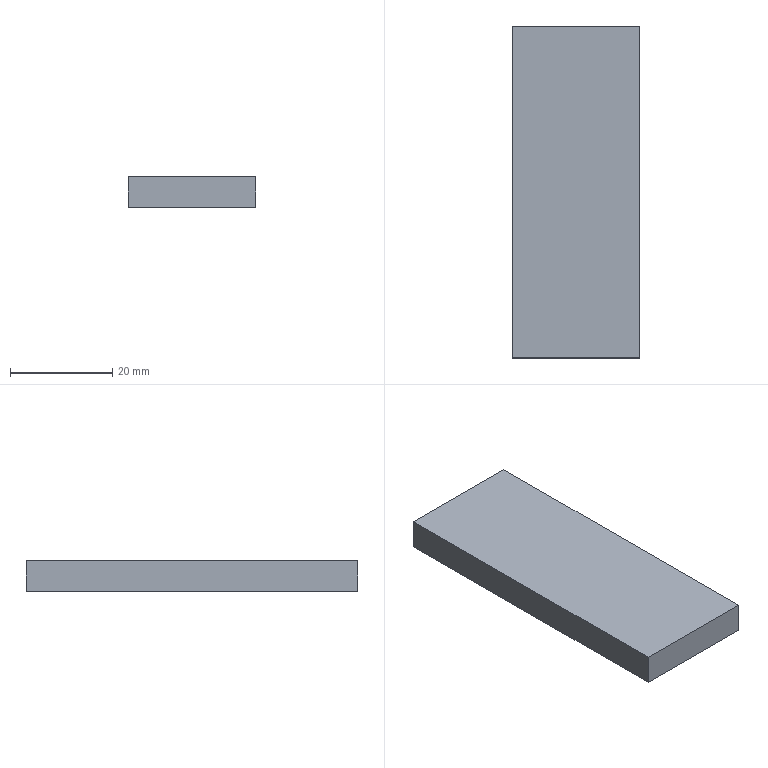Part | STEP file | 09-Steel plate 25x65x6 | 1 solid | 6 faces | box 25 x 65 x 6 mm | volume 9750 mm3 | plane 6
STEP:
#1=CARTESIAN_POINT('',(0.,0.,0.));
#2=DIRECTION('',(0.,0.,1.));
#3=DIRECTION('',(1.,0.,0.));
#4=AXIS2_PLACEMENT_3D('',#1,#2,#3);
#5=CARTESIAN_POINT('',(0.,0.,0.));
#6=VERTEX_POINT('',#5);
#7=CARTESIAN_POINT('',(0.,-65.,0.));
#8=VERTEX_POINT('',#7);
#9=CARTESIAN_POINT('',(0.,0.,0.));
#10=DIRECTION('',(0.,-1.,0.));
#11=VECTOR('',#10,1.);
#12=LINE('',#9,#11);
#13=CARTESIAN_POINT('',(0.,0.,6.));
#14=DIRECTION('',(1.,0.,0.));
#15=DIRECTION('',(0.,1.,0.));
#16=AXIS2_PLACEMENT_3D('',#13,#14,#15);
#17=PLANE('',#16);
#18=CARTESIAN_POINT('',(0.,-6.));
#19=DIRECTION('',(-1.,0.));
#20=VECTOR('',#19,1.);
#21=LINE('',#18,#20);
#22=(GEOMETRIC_REPRESENTATION_CONTEXT(2)PARAMETRIC_REPRESENTATION_CONTEXT()REPRESENTATION_CONTEXT('',''));
#23=DEFINITIONAL_REPRESENTATION('',(#21),#22);
#24=PCURVE('',#17,#23);
#25=CARTESIAN_POINT('',(0.,0.,0.));
#26=DIRECTION('',(0.,0.,1.));
#27=DIRECTION('',(1.,0.,0.));
#28=AXIS2_PLACEMENT_3D('',#25,#26,#27);
#29=PLANE('',#28);
#30=CARTESIAN_POINT('',(0.,0.));
#31=DIRECTION('',(0.,-1.));
#32=VECTOR('',#31,1.);
#33=LINE('',#30,#32);
#34=(GEOMETRIC_REPRESENTATION_CONTEXT(2)PARAMETRIC_REPRESENTATION_CONTEXT()REPRESENTATION_CONTEXT('',''));
#35=DEFINITIONAL_REPRESENTATION('',(#33),#34);
#36=PCURVE('',#29,#35);
#37=SURFACE_CURVE('',#12,(#24,#36),.PCURVE_S1.);
#38=EDGE_CURVE('',#6,#8,#37,.T.);
#39=ORIENTED_EDGE('',*,*,#38,.T.);
#40=CARTESIAN_POINT('',(0.,-65.,6.));
#41=VERTEX_POINT('',#40);
#42=CARTESIAN_POINT('',(0.,-65.,6.));
#43=DIRECTION('',(0.,0.,-1.));
#44=VECTOR('',#43,1.);
#45=LINE('',#42,#44);
#46=CARTESIAN_POINT('',(-65.,0.));
#47=DIRECTION('',(0.,-1.));
#48=VECTOR('',#47,1.);
#49=LINE('',#46,#48);
#50=(GEOMETRIC_REPRESENTATION_CONTEXT(2)PARAMETRIC_REPRESENTATION_CONTEXT()REPRESENTATION_CONTEXT('',''));
#51=DEFINITIONAL_REPRESENTATION('',(#49),#50);
#52=PCURVE('',#17,#51);
#53=CARTESIAN_POINT('',(0.,-65.,6.));
#54=DIRECTION('',(0.,1.,0.));
#55=DIRECTION('',(0.,0.,1.));
#56=AXIS2_PLACEMENT_3D('',#53,#54,#55);
#57=PLANE('',#56);
#58=CARTESIAN_POINT('',(0.,0.));
#59=DIRECTION('',(-1.,0.));
#60=VECTOR('',#59,1.);
#61=LINE('',#58,#60);
#62=(GEOMETRIC_REPRESENTATION_CONTEXT(2)PARAMETRIC_REPRESENTATION_CONTEXT()REPRESENTATION_CONTEXT('',''));
#63=DEFINITIONAL_REPRESENTATION('',(#61),#62);
#64=PCURVE('',#57,#63);
#65=SURFACE_CURVE('',#45,(#52,#64),.PCURVE_S1.);
#66=EDGE_CURVE('',#41,#8,#65,.T.);
#67=ORIENTED_EDGE('',*,*,#66,.F.);
#68=CARTESIAN_POINT('',(0.,0.,6.));
#69=VERTEX_POINT('',#68);
#70=CARTESIAN_POINT('',(0.,0.,6.));
#71=DIRECTION('',(0.,-1.,0.));
#72=VECTOR('',#71,1.);
#73=LINE('',#70,#72);
#74=CARTESIAN_POINT('',(0.,0.));
#75=DIRECTION('',(-1.,0.));
#76=VECTOR('',#75,1.);
#77=LINE('',#74,#76);
#78=(GEOMETRIC_REPRESENTATION_CONTEXT(2)PARAMETRIC_REPRESENTATION_CONTEXT()REPRESENTATION_CONTEXT('',''));
#79=DEFINITIONAL_REPRESENTATION('',(#77),#78);
#80=PCURVE('',#17,#79);
#81=CARTESIAN_POINT('',(0.,0.,6.));
#82=DIRECTION('',(0.,0.,1.));
#83=DIRECTION('',(1.,0.,0.));
#84=AXIS2_PLACEMENT_3D('',#81,#82,#83);
#85=PLANE('',#84);
#86=CARTESIAN_POINT('',(0.,0.));
#87=DIRECTION('',(0.,-1.));
#88=VECTOR('',#87,1.);
#89=LINE('',#86,#88);
#90=(GEOMETRIC_REPRESENTATION_CONTEXT(2)PARAMETRIC_REPRESENTATION_CONTEXT()REPRESENTATION_CONTEXT('',''));
#91=DEFINITIONAL_REPRESENTATION('',(#89),#90);
#92=PCURVE('',#85,#91);
#93=SURFACE_CURVE('',#73,(#80,#92),.PCURVE_S1.);
#94=EDGE_CURVE('',#69,#41,#93,.T.);
#95=ORIENTED_EDGE('',*,*,#94,.F.);
#96=CARTESIAN_POINT('',(0.,0.,6.));
#97=DIRECTION('',(0.,0.,-1.));
#98=VECTOR('',#97,1.);
#99=LINE('',#96,#98);
#100=CARTESIAN_POINT('',(0.,0.));
#101=DIRECTION('',(0.,-1.));
#102=VECTOR('',#101,1.);
#103=LINE('',#100,#102);
#104=(GEOMETRIC_REPRESENTATION_CONTEXT(2)PARAMETRIC_REPRESENTATION_CONTEXT()REPRESENTATION_CONTEXT('',''));
#105=DEFINITIONAL_REPRESENTATION('',(#103),#104);
#106=PCURVE('',#17,#105);
#107=CARTESIAN_POINT('',(0.,0.,6.));
#108=DIRECTION('',(0.,-1.,0.));
#109=DIRECTION('',(0.,0.,-1.));
#110=AXIS2_PLACEMENT_3D('',#107,#108,#109);
#111=PLANE('',#110);
#112=CARTESIAN_POINT('',(0.,0.));
#113=DIRECTION('',(1.,0.));
#114=VECTOR('',#113,1.);
#115=LINE('',#112,#114);
#116=(GEOMETRIC_REPRESENTATION_CONTEXT(2)PARAMETRIC_REPRESENTATION_CONTEXT()REPRESENTATION_CONTEXT('',''));
#117=DEFINITIONAL_REPRESENTATION('',(#115),#116);
#118=PCURVE('',#111,#117);
#119=SURFACE_CURVE('',#99,(#106,#118),.PCURVE_S1.);
#120=EDGE_CURVE('',#69,#6,#119,.T.);
#121=ORIENTED_EDGE('',*,*,#120,.T.);
#122=EDGE_LOOP('',(#39,#67,#95,#121));
#123=FACE_BOUND('',#122,.T.);
#124=ADVANCED_FACE('',(#123),#17,.F.);
#125=CARTESIAN_POINT('',(25.,-65.,0.));
#126=VERTEX_POINT('',#125);
#127=CARTESIAN_POINT('',(0.,-65.,0.));
#128=DIRECTION('',(1.,0.,0.));
#129=VECTOR('',#128,1.);
#130=LINE('',#127,#129);
#131=CARTESIAN_POINT('',(-6.,0.));
#132=DIRECTION('',(0.,1.));
#133=VECTOR('',#132,1.);
#134=LINE('',#131,#133);
#135=(GEOMETRIC_REPRESENTATION_CONTEXT(2)PARAMETRIC_REPRESENTATION_CONTEXT()REPRESENTATION_CONTEXT('',''));
#136=DEFINITIONAL_REPRESENTATION('',(#134),#135);
#137=PCURVE('',#57,#136);
#138=CARTESIAN_POINT('',(0.,-65.));
#139=DIRECTION('',(1.,0.));
#140=VECTOR('',#139,1.);
#141=LINE('',#138,#140);
#142=(GEOMETRIC_REPRESENTATION_CONTEXT(2)PARAMETRIC_REPRESENTATION_CONTEXT()REPRESENTATION_CONTEXT('',''));
#143=DEFINITIONAL_REPRESENTATION('',(#141),#142);
#144=PCURVE('',#29,#143);
#145=SURFACE_CURVE('',#130,(#137,#144),.PCURVE_S1.);
#146=EDGE_CURVE('',#8,#126,#145,.T.);
#147=ORIENTED_EDGE('',*,*,#146,.T.);
#148=CARTESIAN_POINT('',(25.,-65.,6.));
#149=VERTEX_POINT('',#148);
#150=CARTESIAN_POINT('',(25.,-65.,6.));
#151=DIRECTION('',(0.,0.,-1.));
#152=VECTOR('',#151,1.);
#153=LINE('',#150,#152);
#154=CARTESIAN_POINT('',(0.,25.));
#155=DIRECTION('',(-1.,0.));
#156=VECTOR('',#155,1.);
#157=LINE('',#154,#156);
#158=(GEOMETRIC_REPRESENTATION_CONTEXT(2)PARAMETRIC_REPRESENTATION_CONTEXT()REPRESENTATION_CONTEXT('',''));
#159=DEFINITIONAL_REPRESENTATION('',(#157),#158);
#160=PCURVE('',#57,#159);
#161=CARTESIAN_POINT('',(25.,0.,6.));
#162=DIRECTION('',(-1.,0.,0.));
#163=DIRECTION('',(0.,-1.,0.));
#164=AXIS2_PLACEMENT_3D('',#161,#162,#163);
#165=PLANE('',#164);
#166=CARTESIAN_POINT('',(65.,0.));
#167=DIRECTION('',(0.,-1.));
#168=VECTOR('',#167,1.);
#169=LINE('',#166,#168);
#170=(GEOMETRIC_REPRESENTATION_CONTEXT(2)PARAMETRIC_REPRESENTATION_CONTEXT()REPRESENTATION_CONTEXT('',''));
#171=DEFINITIONAL_REPRESENTATION('',(#169),#170);
#172=PCURVE('',#165,#171);
#173=SURFACE_CURVE('',#153,(#160,#172),.PCURVE_S1.);
#174=EDGE_CURVE('',#149,#126,#173,.T.);
#175=ORIENTED_EDGE('',*,*,#174,.F.);
#176=CARTESIAN_POINT('',(0.,-65.,6.));
#177=DIRECTION('',(1.,0.,0.));
#178=VECTOR('',#177,1.);
#179=LINE('',#176,#178);
#180=CARTESIAN_POINT('',(0.,0.));
#181=DIRECTION('',(0.,1.));
#182=VECTOR('',#181,1.);
#183=LINE('',#180,#182);
#184=(GEOMETRIC_REPRESENTATION_CONTEXT(2)PARAMETRIC_REPRESENTATION_CONTEXT()REPRESENTATION_CONTEXT('',''));
#185=DEFINITIONAL_REPRESENTATION('',(#183),#184);
#186=PCURVE('',#57,#185);
#187=CARTESIAN_POINT('',(0.,-65.));
#188=DIRECTION('',(1.,0.));
#189=VECTOR('',#188,1.);
#190=LINE('',#187,#189);
#191=(GEOMETRIC_REPRESENTATION_CONTEXT(2)PARAMETRIC_REPRESENTATION_CONTEXT()REPRESENTATION_CONTEXT('',''));
#192=DEFINITIONAL_REPRESENTATION('',(#190),#191);
#193=PCURVE('',#85,#192);
#194=SURFACE_CURVE('',#179,(#186,#193),.PCURVE_S1.);
#195=EDGE_CURVE('',#41,#149,#194,.T.);
#196=ORIENTED_EDGE('',*,*,#195,.F.);
#197=ORIENTED_EDGE('',*,*,#66,.T.);
#198=EDGE_LOOP('',(#147,#175,#196,#197));
#199=FACE_BOUND('',#198,.T.);
#200=ADVANCED_FACE('',(#199),#57,.F.);
#201=CARTESIAN_POINT('',(25.,0.,0.));
#202=VERTEX_POINT('',#201);
#203=CARTESIAN_POINT('',(25.,0.,0.));
#204=DIRECTION('',(0.,1.,0.));
#205=VECTOR('',#204,1.);
#206=LINE('',#203,#205);
#207=CARTESIAN_POINT('',(0.,-6.));
#208=DIRECTION('',(-1.,0.));
#209=VECTOR('',#208,1.);
#210=LINE('',#207,#209);
#211=(GEOMETRIC_REPRESENTATION_CONTEXT(2)PARAMETRIC_REPRESENTATION_CONTEXT()REPRESENTATION_CONTEXT('',''));
#212=DEFINITIONAL_REPRESENTATION('',(#210),#211);
#213=PCURVE('',#165,#212);
#214=CARTESIAN_POINT('',(25.,0.));
#215=DIRECTION('',(0.,1.));
#216=VECTOR('',#215,1.);
#217=LINE('',#214,#216);
#218=(GEOMETRIC_REPRESENTATION_CONTEXT(2)PARAMETRIC_REPRESENTATION_CONTEXT()REPRESENTATION_CONTEXT('',''));
#219=DEFINITIONAL_REPRESENTATION('',(#217),#218);
#220=PCURVE('',#29,#219);
#221=SURFACE_CURVE('',#206,(#213,#220),.PCURVE_S1.);
#222=EDGE_CURVE('',#126,#202,#221,.T.);
#223=ORIENTED_EDGE('',*,*,#222,.T.);
#224=CARTESIAN_POINT('',(25.,0.,6.));
#225=VERTEX_POINT('',#224);
#226=CARTESIAN_POINT('',(25.,0.,6.));
#227=DIRECTION('',(0.,0.,-1.));
#228=VECTOR('',#227,1.);
#229=LINE('',#226,#228);
#230=CARTESIAN_POINT('',(0.,0.));
#231=DIRECTION('',(0.,-1.));
#232=VECTOR('',#231,1.);
#233=LINE('',#230,#232);
#234=(GEOMETRIC_REPRESENTATION_CONTEXT(2)PARAMETRIC_REPRESENTATION_CONTEXT()REPRESENTATION_CONTEXT('',''));
#235=DEFINITIONAL_REPRESENTATION('',(#233),#234);
#236=PCURVE('',#165,#235);
#237=CARTESIAN_POINT('',(0.,25.));
#238=DIRECTION('',(1.,0.));
#239=VECTOR('',#238,1.);
#240=LINE('',#237,#239);
#241=(GEOMETRIC_REPRESENTATION_CONTEXT(2)PARAMETRIC_REPRESENTATION_CONTEXT()REPRESENTATION_CONTEXT('',''));
#242=DEFINITIONAL_REPRESENTATION('',(#240),#241);
#243=PCURVE('',#111,#242);
#244=SURFACE_CURVE('',#229,(#236,#243),.PCURVE_S1.);
#245=EDGE_CURVE('',#225,#202,#244,.T.);
#246=ORIENTED_EDGE('',*,*,#245,.F.);
#247=CARTESIAN_POINT('',(25.,0.,6.));
#248=DIRECTION('',(0.,1.,0.));
#249=VECTOR('',#248,1.);
#250=LINE('',#247,#249);
#251=CARTESIAN_POINT('',(0.,0.));
#252=DIRECTION('',(-1.,0.));
#253=VECTOR('',#252,1.);
#254=LINE('',#251,#253);
#255=(GEOMETRIC_REPRESENTATION_CONTEXT(2)PARAMETRIC_REPRESENTATION_CONTEXT()REPRESENTATION_CONTEXT('',''));
#256=DEFINITIONAL_REPRESENTATION('',(#254),#255);
#257=PCURVE('',#165,#256);
#258=CARTESIAN_POINT('',(25.,0.));
#259=DIRECTION('',(0.,1.));
#260=VECTOR('',#259,1.);
#261=LINE('',#258,#260);
#262=(GEOMETRIC_REPRESENTATION_CONTEXT(2)PARAMETRIC_REPRESENTATION_CONTEXT()REPRESENTATION_CONTEXT('',''));
#263=DEFINITIONAL_REPRESENTATION('',(#261),#262);
#264=PCURVE('',#85,#263);
#265=SURFACE_CURVE('',#250,(#257,#264),.PCURVE_S1.);
#266=EDGE_CURVE('',#149,#225,#265,.T.);
#267=ORIENTED_EDGE('',*,*,#266,.F.);
#268=ORIENTED_EDGE('',*,*,#174,.T.);
#269=EDGE_LOOP('',(#223,#246,#267,#268));
#270=FACE_BOUND('',#269,.T.);
#271=ADVANCED_FACE('',(#270),#165,.F.);
#272=CARTESIAN_POINT('',(0.,0.,0.));
#273=DIRECTION('',(-1.,0.,0.));
#274=VECTOR('',#273,1.);
#275=LINE('',#272,#274);
#276=CARTESIAN_POINT('',(6.,0.));
#277=DIRECTION('',(0.,-1.));
#278=VECTOR('',#277,1.);
#279=LINE('',#276,#278);
#280=(GEOMETRIC_REPRESENTATION_CONTEXT(2)PARAMETRIC_REPRESENTATION_CONTEXT()REPRESENTATION_CONTEXT('',''));
#281=DEFINITIONAL_REPRESENTATION('',(#279),#280);
#282=PCURVE('',#111,#281);
#283=CARTESIAN_POINT('',(0.,0.));
#284=DIRECTION('',(-1.,0.));
#285=VECTOR('',#284,1.);
#286=LINE('',#283,#285);
#287=(GEOMETRIC_REPRESENTATION_CONTEXT(2)PARAMETRIC_REPRESENTATION_CONTEXT()REPRESENTATION_CONTEXT('',''));
#288=DEFINITIONAL_REPRESENTATION('',(#286),#287);
#289=PCURVE('',#29,#288);
#290=SURFACE_CURVE('',#275,(#282,#289),.PCURVE_S1.);
#291=EDGE_CURVE('',#202,#6,#290,.T.);
#292=ORIENTED_EDGE('',*,*,#291,.T.);
#293=ORIENTED_EDGE('',*,*,#120,.F.);
#294=CARTESIAN_POINT('',(0.,0.,6.));
#295=DIRECTION('',(-1.,0.,0.));
#296=VECTOR('',#295,1.);
#297=LINE('',#294,#296);
#298=CARTESIAN_POINT('',(0.,0.));
#299=DIRECTION('',(0.,-1.));
#300=VECTOR('',#299,1.);
#301=LINE('',#298,#300);
#302=(GEOMETRIC_REPRESENTATION_CONTEXT(2)PARAMETRIC_REPRESENTATION_CONTEXT()REPRESENTATION_CONTEXT('',''));
#303=DEFINITIONAL_REPRESENTATION('',(#301),#302);
#304=PCURVE('',#111,#303);
#305=CARTESIAN_POINT('',(0.,0.));
#306=DIRECTION('',(-1.,0.));
#307=VECTOR('',#306,1.);
#308=LINE('',#305,#307);
#309=(GEOMETRIC_REPRESENTATION_CONTEXT(2)PARAMETRIC_REPRESENTATION_CONTEXT()REPRESENTATION_CONTEXT('',''));
#310=DEFINITIONAL_REPRESENTATION('',(#308),#309);
#311=PCURVE('',#85,#310);
#312=SURFACE_CURVE('',#297,(#304,#311),.PCURVE_S1.);
#313=EDGE_CURVE('',#225,#69,#312,.T.);
#314=ORIENTED_EDGE('',*,*,#313,.F.);
#315=ORIENTED_EDGE('',*,*,#245,.T.);
#316=EDGE_LOOP('',(#292,#293,#314,#315));
#317=FACE_BOUND('',#316,.T.);
#318=ADVANCED_FACE('',(#317),#111,.F.);
#319=ORIENTED_EDGE('',*,*,#94,.T.);
#320=ORIENTED_EDGE('',*,*,#195,.T.);
#321=ORIENTED_EDGE('',*,*,#266,.T.);
#322=ORIENTED_EDGE('',*,*,#313,.T.);
#323=EDGE_LOOP('',(#319,#320,#321,#322));
#324=FACE_BOUND('',#323,.T.);
#325=ADVANCED_FACE('',(#324),#85,.T.);
#326=ORIENTED_EDGE('',*,*,#38,.F.);
#327=ORIENTED_EDGE('',*,*,#291,.F.);
#328=ORIENTED_EDGE('',*,*,#222,.F.);
#329=ORIENTED_EDGE('',*,*,#146,.F.);
#330=EDGE_LOOP('',(#326,#327,#328,#329));
#331=FACE_BOUND('',#330,.T.);
#332=ADVANCED_FACE('',(#331),#29,.F.);
#333=CLOSED_SHELL('',(#124,#200,#271,#318,#325,#332));
#334=MANIFOLD_SOLID_BREP('',#333);
#335=(LENGTH_UNIT()NAMED_UNIT(*)SI_UNIT(.MILLI.,.METRE.));
#336=UNCERTAINTY_MEASURE_WITH_UNIT(LENGTH_MEASURE(0.0000001),#335,'','');
#337=(NAMED_UNIT(*)PLANE_ANGLE_UNIT()SI_UNIT($,.RADIAN.));
#338=(NAMED_UNIT(*)SI_UNIT($,.STERADIAN.)SOLID_ANGLE_UNIT());
#339=(GEOMETRIC_REPRESENTATION_CONTEXT(3)GLOBAL_UNCERTAINTY_ASSIGNED_CONTEXT((#336))GLOBAL_UNIT_ASSIGNED_CONTEXT((#335,#337,#338))REPRESENTATION_CONTEXT('',''));
#340=ADVANCED_BREP_SHAPE_REPRESENTATION('',(#4,#334),#339);